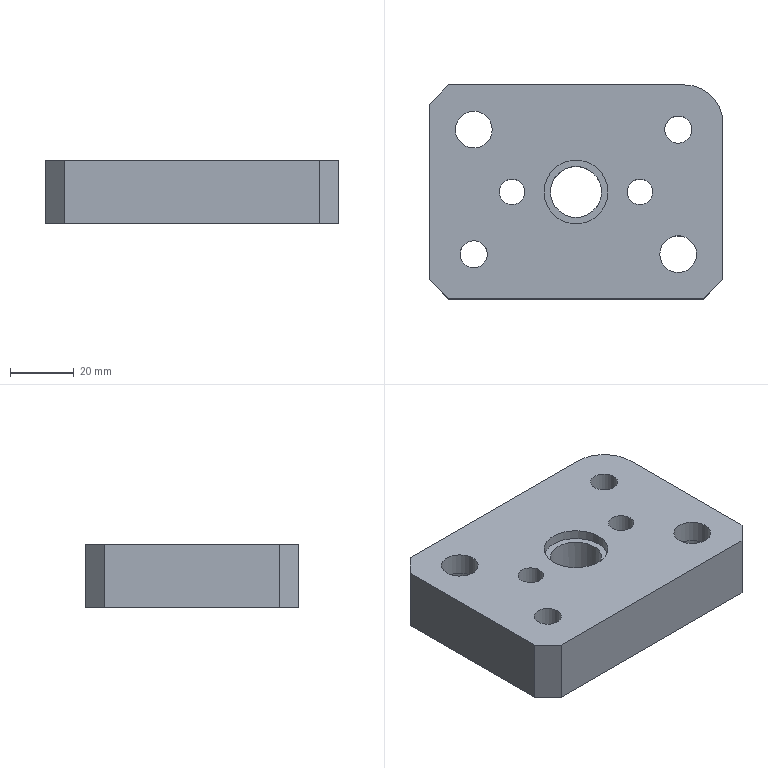Part | STEP file | lll_id594_x_t | 1 solid | 23 faces | box 92 x 67 x 20 mm | volume 104861 mm3 | plane 12 | cylinder 11 | commonest cylinder face diameters 8 x2 8.505 x2 11.509 x2 18.007 x2 16 x1 20 x1
STEP:
#1=CARTESIAN_POINT('',(994.747,-319.5,2.5));
#2=VERTEX_POINT('',#1);
#3=CARTESIAN_POINT('',(999.,-319.5,2.5));
#4=DIRECTION('',(0.,0.,-1.));
#5=DIRECTION('',(-1.,0.,0.));
#6=AXIS2_PLACEMENT_3D('',#3,#4,#5);
#7=CIRCLE('',#6,4.253);
#8=EDGE_CURVE('',#2,#2,#7,.T.);
#9=ORIENTED_EDGE('',*,*,#8,.F.);
#10=EDGE_LOOP('',(#9));
#11=FACE_BOUND('',#10,.T.);
#12=CARTESIAN_POINT('',(1072.003,-319.5,2.5));
#13=VERTEX_POINT('',#12);
#14=CARTESIAN_POINT('',(1063.,-319.5,2.5));
#15=DIRECTION('',(0.,0.,1.));
#16=DIRECTION('',(1.,0.,0.));
#17=AXIS2_PLACEMENT_3D('',#14,#15,#16);
#18=CIRCLE('',#17,9.004);
#19=EDGE_CURVE('',#13,#13,#18,.T.);
#20=ORIENTED_EDGE('',*,*,#19,.T.);
#21=EDGE_LOOP('',(#20));
#22=FACE_BOUND('',#21,.T.);
#23=CARTESIAN_POINT('',(1023.,-300.,2.5));
#24=VERTEX_POINT('',#23);
#25=CARTESIAN_POINT('',(1031.,-300.,2.5));
#26=DIRECTION('',(0.,0.,-1.));
#27=DIRECTION('',(-1.,0.,0.));
#28=AXIS2_PLACEMENT_3D('',#25,#26,#27);
#29=CIRCLE('',#28,8.);
#30=EDGE_CURVE('',#24,#24,#29,.T.);
#31=ORIENTED_EDGE('',*,*,#30,.F.);
#32=EDGE_LOOP('',(#31));
#33=FACE_BOUND('',#32,.T.);
#34=CARTESIAN_POINT('',(1047.,-300.,2.5));
#35=VERTEX_POINT('',#34);
#36=CARTESIAN_POINT('',(1051.,-300.,2.5));
#37=DIRECTION('',(0.,0.,-1.));
#38=DIRECTION('',(-1.,0.,0.));
#39=AXIS2_PLACEMENT_3D('',#36,#37,#38);
#40=CIRCLE('',#39,4.);
#41=EDGE_CURVE('',#35,#35,#40,.T.);
#42=ORIENTED_EDGE('',*,*,#41,.F.);
#43=EDGE_LOOP('',(#42));
#44=FACE_BOUND('',#43,.T.);
#45=CARTESIAN_POINT('',(1007.,-300.,2.5));
#46=VERTEX_POINT('',#45);
#47=CARTESIAN_POINT('',(1011.,-300.,2.5));
#48=DIRECTION('',(0.,0.,-1.));
#49=DIRECTION('',(-1.,0.,0.));
#50=AXIS2_PLACEMENT_3D('',#47,#48,#49);
#51=CIRCLE('',#50,4.);
#52=EDGE_CURVE('',#46,#46,#51,.T.);
#53=ORIENTED_EDGE('',*,*,#52,.F.);
#54=EDGE_LOOP('',(#53));
#55=FACE_BOUND('',#54,.T.);
#56=CARTESIAN_POINT('',(1065.,-266.5,2.5));
#57=VERTEX_POINT('',#56);
#58=CARTESIAN_POINT('',(991.,-266.5,2.5));
#59=VERTEX_POINT('',#58);
#60=CARTESIAN_POINT('',(1031.,-266.5,2.5));
#61=DIRECTION('',(-1.,0.,0.));
#62=VECTOR('',#61,1.);
#63=LINE('',#60,#62);
#64=EDGE_CURVE('',#57,#59,#63,.T.);
#65=ORIENTED_EDGE('',*,*,#64,.F.);
#66=CARTESIAN_POINT('',(1077.,-278.5,2.5));
#67=VERTEX_POINT('',#66);
#68=CARTESIAN_POINT('',(1065.,-278.5,2.5));
#69=DIRECTION('',(0.,0.,-1.));
#70=DIRECTION('',(-1.,0.,0.));
#71=AXIS2_PLACEMENT_3D('',#68,#69,#70);
#72=CIRCLE('',#71,12.);
#73=EDGE_CURVE('',#57,#67,#72,.T.);
#74=ORIENTED_EDGE('',*,*,#73,.T.);
#75=CARTESIAN_POINT('',(1077.,-327.5,2.5));
#76=VERTEX_POINT('',#75);
#77=CARTESIAN_POINT('',(1077.,-300.,2.5));
#78=DIRECTION('',(0.,1.,0.));
#79=VECTOR('',#78,1.);
#80=LINE('',#77,#79);
#81=EDGE_CURVE('',#76,#67,#80,.T.);
#82=ORIENTED_EDGE('',*,*,#81,.F.);
#83=CARTESIAN_POINT('',(1071.,-333.5,2.5));
#84=VERTEX_POINT('',#83);
#85=CARTESIAN_POINT('',(915.125,-489.375,2.5));
#86=DIRECTION('',(-0.7071,-0.7071,0.));
#87=VECTOR('',#86,1.);
#88=LINE('',#85,#87);
#89=EDGE_CURVE('',#76,#84,#88,.T.);
#90=ORIENTED_EDGE('',*,*,#89,.T.);
#91=CARTESIAN_POINT('',(991.,-333.5,2.5));
#92=VERTEX_POINT('',#91);
#93=CARTESIAN_POINT('',(1031.,-333.5,2.5));
#94=DIRECTION('',(1.,0.,0.));
#95=VECTOR('',#94,1.);
#96=LINE('',#93,#95);
#97=EDGE_CURVE('',#92,#84,#96,.T.);
#98=ORIENTED_EDGE('',*,*,#97,.F.);
#99=CARTESIAN_POINT('',(985.,-327.5,2.5));
#100=VERTEX_POINT('',#99);
#101=CARTESIAN_POINT('',(849.875,-192.375,2.5));
#102=DIRECTION('',(-0.7071,0.7071,0.));
#103=VECTOR('',#102,1.);
#104=LINE('',#101,#103);
#105=EDGE_CURVE('',#92,#100,#104,.T.);
#106=ORIENTED_EDGE('',*,*,#105,.T.);
#107=CARTESIAN_POINT('',(985.,-272.5,2.5));
#108=VERTEX_POINT('',#107);
#109=CARTESIAN_POINT('',(985.,-300.,2.5));
#110=DIRECTION('',(0.,-1.,0.));
#111=VECTOR('',#110,1.);
#112=LINE('',#109,#111);
#113=EDGE_CURVE('',#108,#100,#112,.T.);
#114=ORIENTED_EDGE('',*,*,#113,.F.);
#115=CARTESIAN_POINT('',(841.625,-415.875,2.5));
#116=DIRECTION('',(0.7071,0.7071,0.));
#117=VECTOR('',#116,1.);
#118=LINE('',#115,#117);
#119=EDGE_CURVE('',#108,#59,#118,.T.);
#120=ORIENTED_EDGE('',*,*,#119,.T.);
#121=EDGE_LOOP('',(#65,#74,#82,#90,#98,#106,#114,#120));
#122=FACE_BOUND('',#121,.T.);
#123=CARTESIAN_POINT('',(1058.747,-280.5,2.5));
#124=VERTEX_POINT('',#123);
#125=CARTESIAN_POINT('',(1063.,-280.5,2.5));
#126=DIRECTION('',(0.,0.,-1.));
#127=DIRECTION('',(-1.,0.,0.));
#128=AXIS2_PLACEMENT_3D('',#125,#126,#127);
#129=CIRCLE('',#128,4.253);
#130=EDGE_CURVE('',#124,#124,#129,.T.);
#131=ORIENTED_EDGE('',*,*,#130,.F.);
#132=EDGE_LOOP('',(#131));
#133=FACE_BOUND('',#132,.T.);
#134=CARTESIAN_POINT('',(1008.003,-280.5,2.5));
#135=VERTEX_POINT('',#134);
#136=CARTESIAN_POINT('',(999.,-280.5,2.5));
#137=DIRECTION('',(0.,0.,1.));
#138=DIRECTION('',(1.,0.,0.));
#139=AXIS2_PLACEMENT_3D('',#136,#137,#138);
#140=CIRCLE('',#139,9.004);
#141=EDGE_CURVE('',#135,#135,#140,.T.);
#142=ORIENTED_EDGE('',*,*,#141,.T.);
#143=EDGE_LOOP('',(#142));
#144=FACE_BOUND('',#143,.T.);
#145=CARTESIAN_POINT('',(734.,-308.25,2.5));
#146=DIRECTION('',(0.,0.,-1.));
#147=DIRECTION('',(1.,0.,0.));
#148=AXIS2_PLACEMENT_3D('',#145,#146,#147);
#149=PLANE('',#148);
#150=ADVANCED_FACE('',(#11,#22,#33,#44,#55,#122,#133,#144),#149,.T.);
#151=CARTESIAN_POINT('',(1003.252,-319.5,22.5));
#152=VERTEX_POINT('',#151);
#153=CARTESIAN_POINT('',(999.,-319.5,22.5));
#154=DIRECTION('',(0.,0.,1.));
#155=DIRECTION('',(1.,0.,0.));
#156=AXIS2_PLACEMENT_3D('',#153,#154,#155);
#157=CIRCLE('',#156,4.253);
#158=EDGE_CURVE('',#152,#152,#157,.T.);
#159=ORIENTED_EDGE('',*,*,#158,.F.);
#160=EDGE_LOOP('',(#159));
#161=FACE_BOUND('',#160,.T.);
#162=CARTESIAN_POINT('',(1004.754,-280.5,22.5));
#163=VERTEX_POINT('',#162);
#164=CARTESIAN_POINT('',(999.,-280.5,22.5));
#165=DIRECTION('',(0.,0.,1.));
#166=DIRECTION('',(1.,0.,0.));
#167=AXIS2_PLACEMENT_3D('',#164,#165,#166);
#168=CIRCLE('',#167,5.755);
#169=EDGE_CURVE('',#163,#163,#168,.T.);
#170=ORIENTED_EDGE('',*,*,#169,.F.);
#171=EDGE_LOOP('',(#170));
#172=FACE_BOUND('',#171,.T.);
#173=CARTESIAN_POINT('',(1067.252,-280.5,22.5));
#174=VERTEX_POINT('',#173);
#175=CARTESIAN_POINT('',(1063.,-280.5,22.5));
#176=DIRECTION('',(0.,0.,1.));
#177=DIRECTION('',(1.,0.,0.));
#178=AXIS2_PLACEMENT_3D('',#175,#176,#177);
#179=CIRCLE('',#178,4.253);
#180=EDGE_CURVE('',#174,#174,#179,.T.);
#181=ORIENTED_EDGE('',*,*,#180,.F.);
#182=EDGE_LOOP('',(#181));
#183=FACE_BOUND('',#182,.T.);
#184=CARTESIAN_POINT('',(1068.754,-319.5,22.5));
#185=VERTEX_POINT('',#184);
#186=CARTESIAN_POINT('',(1063.,-319.5,22.5));
#187=DIRECTION('',(0.,0.,1.));
#188=DIRECTION('',(1.,0.,0.));
#189=AXIS2_PLACEMENT_3D('',#186,#187,#188);
#190=CIRCLE('',#189,5.755);
#191=EDGE_CURVE('',#185,#185,#190,.T.);
#192=ORIENTED_EDGE('',*,*,#191,.F.);
#193=EDGE_LOOP('',(#192));
#194=FACE_BOUND('',#193,.T.);
#195=CARTESIAN_POINT('',(1077.,-278.5,22.5));
#196=VERTEX_POINT('',#195);
#197=CARTESIAN_POINT('',(1077.,-327.5,22.5));
#198=VERTEX_POINT('',#197);
#199=CARTESIAN_POINT('',(1077.,-300.,22.5));
#200=DIRECTION('',(0.,-1.,0.));
#201=VECTOR('',#200,1.);
#202=LINE('',#199,#201);
#203=EDGE_CURVE('',#196,#198,#202,.T.);
#204=ORIENTED_EDGE('',*,*,#203,.F.);
#205=CARTESIAN_POINT('',(1065.,-266.5,22.5));
#206=VERTEX_POINT('',#205);
#207=CARTESIAN_POINT('',(1065.,-278.5,22.5));
#208=DIRECTION('',(0.,0.,1.));
#209=DIRECTION('',(1.,0.,0.));
#210=AXIS2_PLACEMENT_3D('',#207,#208,#209);
#211=CIRCLE('',#210,12.);
#212=EDGE_CURVE('',#196,#206,#211,.T.);
#213=ORIENTED_EDGE('',*,*,#212,.T.);
#214=CARTESIAN_POINT('',(991.,-266.5,22.5));
#215=VERTEX_POINT('',#214);
#216=CARTESIAN_POINT('',(1031.,-266.5,22.5));
#217=DIRECTION('',(1.,0.,0.));
#218=VECTOR('',#217,1.);
#219=LINE('',#216,#218);
#220=EDGE_CURVE('',#215,#206,#219,.T.);
#221=ORIENTED_EDGE('',*,*,#220,.F.);
#222=CARTESIAN_POINT('',(985.,-272.5,22.5));
#223=VERTEX_POINT('',#222);
#224=CARTESIAN_POINT('',(841.625,-415.875,22.5));
#225=DIRECTION('',(-0.7071,-0.7071,0.));
#226=VECTOR('',#225,1.);
#227=LINE('',#224,#226);
#228=EDGE_CURVE('',#215,#223,#227,.T.);
#229=ORIENTED_EDGE('',*,*,#228,.T.);
#230=CARTESIAN_POINT('',(985.,-327.5,22.5));
#231=VERTEX_POINT('',#230);
#232=CARTESIAN_POINT('',(985.,-300.,22.5));
#233=DIRECTION('',(0.,1.,0.));
#234=VECTOR('',#233,1.);
#235=LINE('',#232,#234);
#236=EDGE_CURVE('',#231,#223,#235,.T.);
#237=ORIENTED_EDGE('',*,*,#236,.F.);
#238=CARTESIAN_POINT('',(991.,-333.5,22.5));
#239=VERTEX_POINT('',#238);
#240=CARTESIAN_POINT('',(849.875,-192.375,22.5));
#241=DIRECTION('',(0.7071,-0.7071,0.));
#242=VECTOR('',#241,1.);
#243=LINE('',#240,#242);
#244=EDGE_CURVE('',#231,#239,#243,.T.);
#245=ORIENTED_EDGE('',*,*,#244,.T.);
#246=CARTESIAN_POINT('',(1071.,-333.5,22.5));
#247=VERTEX_POINT('',#246);
#248=CARTESIAN_POINT('',(1031.,-333.5,22.5));
#249=DIRECTION('',(-1.,0.,0.));
#250=VECTOR('',#249,1.);
#251=LINE('',#248,#250);
#252=EDGE_CURVE('',#247,#239,#251,.T.);
#253=ORIENTED_EDGE('',*,*,#252,.F.);
#254=CARTESIAN_POINT('',(915.125,-489.375,22.5));
#255=DIRECTION('',(0.7071,0.7071,0.));
#256=VECTOR('',#255,1.);
#257=LINE('',#254,#256);
#258=EDGE_CURVE('',#247,#198,#257,.T.);
#259=ORIENTED_EDGE('',*,*,#258,.T.);
#260=EDGE_LOOP('',(#204,#213,#221,#229,#237,#245,#253,#259));
#261=FACE_BOUND('',#260,.T.);
#262=CARTESIAN_POINT('',(1041.,-300.,22.5));
#263=VERTEX_POINT('',#262);
#264=CARTESIAN_POINT('',(1031.,-300.,22.5));
#265=DIRECTION('',(0.,0.,-1.));
#266=DIRECTION('',(1.,0.,0.));
#267=AXIS2_PLACEMENT_3D('',#264,#265,#266);
#268=CIRCLE('',#267,10.);
#269=EDGE_CURVE('',#263,#263,#268,.T.);
#270=ORIENTED_EDGE('',*,*,#269,.T.);
#271=EDGE_LOOP('',(#270));
#272=FACE_BOUND('',#271,.T.);
#273=CARTESIAN_POINT('',(1015.,-300.,22.5));
#274=VERTEX_POINT('',#273);
#275=CARTESIAN_POINT('',(1011.,-300.,22.5));
#276=DIRECTION('',(0.,0.,1.));
#277=DIRECTION('',(1.,0.,0.));
#278=AXIS2_PLACEMENT_3D('',#275,#276,#277);
#279=CIRCLE('',#278,4.);
#280=EDGE_CURVE('',#274,#274,#279,.T.);
#281=ORIENTED_EDGE('',*,*,#280,.F.);
#282=EDGE_LOOP('',(#281));
#283=FACE_BOUND('',#282,.T.);
#284=CARTESIAN_POINT('',(1055.,-300.,22.5));
#285=VERTEX_POINT('',#284);
#286=CARTESIAN_POINT('',(1051.,-300.,22.5));
#287=DIRECTION('',(0.,0.,1.));
#288=DIRECTION('',(1.,0.,0.));
#289=AXIS2_PLACEMENT_3D('',#286,#287,#288);
#290=CIRCLE('',#289,4.);
#291=EDGE_CURVE('',#285,#285,#290,.T.);
#292=ORIENTED_EDGE('',*,*,#291,.F.);
#293=EDGE_LOOP('',(#292));
#294=FACE_BOUND('',#293,.T.);
#295=CARTESIAN_POINT('',(734.,-308.25,22.5));
#296=DIRECTION('',(0.,0.,1.));
#297=DIRECTION('',(-1.,0.,0.));
#298=AXIS2_PLACEMENT_3D('',#295,#296,#297);
#299=PLANE('',#298);
#300=ADVANCED_FACE('',(#161,#172,#183,#194,#261,#272,#283,#294),#299,.T.);
#301=ORIENTED_EDGE('',*,*,#81,.T.);
#302=CARTESIAN_POINT('',(1077.,-278.5,-36.5));
#303=DIRECTION('',(0.,0.,1.));
#304=VECTOR('',#303,1.);
#305=LINE('',#302,#304);
#306=EDGE_CURVE('',#67,#196,#305,.T.);
#307=ORIENTED_EDGE('',*,*,#306,.T.);
#308=ORIENTED_EDGE('',*,*,#203,.T.);
#309=CARTESIAN_POINT('',(1077.,-327.5,-36.5));
#310=DIRECTION('',(0.,0.,-1.));
#311=VECTOR('',#310,1.);
#312=LINE('',#309,#311);
#313=EDGE_CURVE('',#198,#76,#312,.T.);
#314=ORIENTED_EDGE('',*,*,#313,.T.);
#315=EDGE_LOOP('',(#301,#307,#308,#314));
#316=FACE_OUTER_BOUND('',#315,.T.);
#317=CARTESIAN_POINT('',(1077.,-300.,-36.5));
#318=DIRECTION('',(1.,0.,0.));
#319=DIRECTION('',(0.,0.,-1.));
#320=AXIS2_PLACEMENT_3D('',#317,#318,#319);
#321=PLANE('',#320);
#322=ADVANCED_FACE('',(#316),#321,.T.);
#323=ORIENTED_EDGE('',*,*,#252,.T.);
#324=CARTESIAN_POINT('',(991.,-333.5,-36.5));
#325=DIRECTION('',(0.,0.,-1.));
#326=VECTOR('',#325,1.);
#327=LINE('',#324,#326);
#328=EDGE_CURVE('',#239,#92,#327,.T.);
#329=ORIENTED_EDGE('',*,*,#328,.T.);
#330=ORIENTED_EDGE('',*,*,#97,.T.);
#331=CARTESIAN_POINT('',(1071.,-333.5,-36.5));
#332=DIRECTION('',(0.,0.,1.));
#333=VECTOR('',#332,1.);
#334=LINE('',#331,#333);
#335=EDGE_CURVE('',#84,#247,#334,.T.);
#336=ORIENTED_EDGE('',*,*,#335,.T.);
#337=EDGE_LOOP('',(#323,#329,#330,#336));
#338=FACE_OUTER_BOUND('',#337,.T.);
#339=CARTESIAN_POINT('',(1031.,-333.5,-36.5));
#340=DIRECTION('',(0.,-1.,0.));
#341=DIRECTION('',(0.,0.,-1.));
#342=AXIS2_PLACEMENT_3D('',#339,#340,#341);
#343=PLANE('',#342);
#344=ADVANCED_FACE('',(#338),#343,.T.);
#345=ORIENTED_EDGE('',*,*,#113,.T.);
#346=CARTESIAN_POINT('',(985.,-327.5,-36.5));
#347=DIRECTION('',(0.,0.,1.));
#348=VECTOR('',#347,1.);
#349=LINE('',#346,#348);
#350=EDGE_CURVE('',#100,#231,#349,.T.);
#351=ORIENTED_EDGE('',*,*,#350,.T.);
#352=ORIENTED_EDGE('',*,*,#236,.T.);
#353=CARTESIAN_POINT('',(985.,-272.5,-36.5));
#354=DIRECTION('',(0.,0.,-1.));
#355=VECTOR('',#354,1.);
#356=LINE('',#353,#355);
#357=EDGE_CURVE('',#223,#108,#356,.T.);
#358=ORIENTED_EDGE('',*,*,#357,.T.);
#359=EDGE_LOOP('',(#345,#351,#352,#358));
#360=FACE_OUTER_BOUND('',#359,.T.);
#361=CARTESIAN_POINT('',(985.,-300.,-36.5));
#362=DIRECTION('',(-1.,0.,0.));
#363=DIRECTION('',(0.,0.,1.));
#364=AXIS2_PLACEMENT_3D('',#361,#362,#363);
#365=PLANE('',#364);
#366=ADVANCED_FACE('',(#360),#365,.T.);
#367=ORIENTED_EDGE('',*,*,#220,.T.);
#368=CARTESIAN_POINT('',(1065.,-266.5,-36.5));
#369=DIRECTION('',(0.,0.,-1.));
#370=VECTOR('',#369,1.);
#371=LINE('',#368,#370);
#372=EDGE_CURVE('',#206,#57,#371,.T.);
#373=ORIENTED_EDGE('',*,*,#372,.T.);
#374=ORIENTED_EDGE('',*,*,#64,.T.);
#375=CARTESIAN_POINT('',(991.,-266.5,-36.5));
#376=DIRECTION('',(0.,0.,1.));
#377=VECTOR('',#376,1.);
#378=LINE('',#375,#377);
#379=EDGE_CURVE('',#59,#215,#378,.T.);
#380=ORIENTED_EDGE('',*,*,#379,.T.);
#381=EDGE_LOOP('',(#367,#373,#374,#380));
#382=FACE_OUTER_BOUND('',#381,.T.);
#383=CARTESIAN_POINT('',(1031.,-266.5,-36.5));
#384=DIRECTION('',(0.,1.,0.));
#385=DIRECTION('',(0.,0.,1.));
#386=AXIS2_PLACEMENT_3D('',#383,#384,#385);
#387=PLANE('',#386);
#388=ADVANCED_FACE('',(#382),#387,.T.);
#389=ORIENTED_EDGE('',*,*,#52,.T.);
#390=EDGE_LOOP('',(#389));
#391=FACE_BOUND('',#390,.T.);
#392=ORIENTED_EDGE('',*,*,#280,.T.);
#393=EDGE_LOOP('',(#392));
#394=FACE_BOUND('',#393,.T.);
#395=CARTESIAN_POINT('',(1011.,-300.,19.5));
#396=DIRECTION('',(0.,0.,-1.));
#397=DIRECTION('',(0.,1.,0.));
#398=AXIS2_PLACEMENT_3D('',#395,#396,#397);
#399=CYLINDRICAL_SURFACE('',#398,4.);
#400=ADVANCED_FACE('',(#391,#394),#399,.F.);
#401=ORIENTED_EDGE('',*,*,#41,.T.);
#402=EDGE_LOOP('',(#401));
#403=FACE_BOUND('',#402,.T.);
#404=ORIENTED_EDGE('',*,*,#291,.T.);
#405=EDGE_LOOP('',(#404));
#406=FACE_BOUND('',#405,.T.);
#407=CARTESIAN_POINT('',(1051.,-300.,19.5));
#408=DIRECTION('',(0.,0.,-1.));
#409=DIRECTION('',(0.,-1.,0.));
#410=AXIS2_PLACEMENT_3D('',#407,#408,#409);
#411=CYLINDRICAL_SURFACE('',#410,4.);
#412=ADVANCED_FACE('',(#403,#406),#411,.F.);
#413=CARTESIAN_POINT('',(1021.,-300.,19.5));
#414=VERTEX_POINT('',#413);
#415=CARTESIAN_POINT('',(1031.,-300.,19.5));
#416=DIRECTION('',(0.,0.,-1.));
#417=DIRECTION('',(-1.,0.,0.));
#418=AXIS2_PLACEMENT_3D('',#415,#416,#417);
#419=CIRCLE('',#418,10.);
#420=EDGE_CURVE('',#414,#414,#419,.T.);
#421=ORIENTED_EDGE('',*,*,#420,.T.);
#422=EDGE_LOOP('',(#421));
#423=FACE_BOUND('',#422,.T.);
#424=ORIENTED_EDGE('',*,*,#269,.F.);
#425=EDGE_LOOP('',(#424));
#426=FACE_BOUND('',#425,.T.);
#427=CARTESIAN_POINT('',(1031.,-300.,22.5));
#428=DIRECTION('',(0.,0.,-1.));
#429=DIRECTION('',(0.,1.,0.));
#430=AXIS2_PLACEMENT_3D('',#427,#428,#429);
#431=CYLINDRICAL_SURFACE('',#430,10.);
#432=ADVANCED_FACE('',(#423,#426),#431,.F.);
#433=CARTESIAN_POINT('',(1031.,-292.,19.5));
#434=VERTEX_POINT('',#433);
#435=CARTESIAN_POINT('',(1031.,-300.,19.5));
#436=DIRECTION('',(0.,0.,1.));
#437=DIRECTION('',(0.,1.,0.));
#438=AXIS2_PLACEMENT_3D('',#435,#436,#437);
#439=CIRCLE('',#438,8.);
#440=EDGE_CURVE('',#434,#434,#439,.T.);
#441=ORIENTED_EDGE('',*,*,#440,.F.);
#442=EDGE_LOOP('',(#441));
#443=FACE_BOUND('',#442,.T.);
#444=ORIENTED_EDGE('',*,*,#420,.F.);
#445=EDGE_LOOP('',(#444));
#446=FACE_BOUND('',#445,.T.);
#447=CARTESIAN_POINT('',(1031.,-300.,19.5));
#448=DIRECTION('',(0.,0.,-1.));
#449=DIRECTION('',(0.,1.,0.));
#450=AXIS2_PLACEMENT_3D('',#447,#448,#449);
#451=PLANE('',#450);
#452=ADVANCED_FACE('',(#443,#446),#451,.F.);
#453=ORIENTED_EDGE('',*,*,#30,.T.);
#454=EDGE_LOOP('',(#453));
#455=FACE_BOUND('',#454,.T.);
#456=ORIENTED_EDGE('',*,*,#440,.T.);
#457=EDGE_LOOP('',(#456));
#458=FACE_BOUND('',#457,.T.);
#459=CARTESIAN_POINT('',(1031.,-300.,15.5));
#460=DIRECTION('',(0.,0.,-1.));
#461=DIRECTION('',(0.,1.,0.));
#462=AXIS2_PLACEMENT_3D('',#459,#460,#461);
#463=CYLINDRICAL_SURFACE('',#462,8.);
#464=ADVANCED_FACE('',(#455,#458),#463,.F.);
#465=ORIENTED_EDGE('',*,*,#191,.T.);
#466=EDGE_LOOP('',(#465));
#467=FACE_BOUND('',#466,.T.);
#468=CARTESIAN_POINT('',(1068.754,-319.5,15.5));
#469=VERTEX_POINT('',#468);
#470=CARTESIAN_POINT('',(1063.,-319.5,15.5));
#471=DIRECTION('',(0.,0.,1.));
#472=DIRECTION('',(1.,0.,0.));
#473=AXIS2_PLACEMENT_3D('',#470,#471,#472);
#474=CIRCLE('',#473,5.755);
#475=EDGE_CURVE('',#469,#469,#474,.T.);
#476=ORIENTED_EDGE('',*,*,#475,.F.);
#477=EDGE_LOOP('',(#476));
#478=FACE_BOUND('',#477,.T.);
#479=CARTESIAN_POINT('',(1063.,-319.5,-2.5));
#480=DIRECTION('',(0.,0.,1.));
#481=DIRECTION('',(1.,0.,0.));
#482=AXIS2_PLACEMENT_3D('',#479,#480,#481);
#483=CYLINDRICAL_SURFACE('',#482,5.755);
#484=ADVANCED_FACE('',(#467,#478),#483,.F.);
#485=ORIENTED_EDGE('',*,*,#475,.T.);
#486=EDGE_LOOP('',(#485));
#487=FACE_BOUND('',#486,.T.);
#488=CARTESIAN_POINT('',(1072.003,-319.5,15.5));
#489=VERTEX_POINT('',#488);
#490=CARTESIAN_POINT('',(1063.,-319.5,15.5));
#491=DIRECTION('',(0.,0.,1.));
#492=DIRECTION('',(1.,0.,0.));
#493=AXIS2_PLACEMENT_3D('',#490,#491,#492);
#494=CIRCLE('',#493,9.004);
#495=EDGE_CURVE('',#489,#489,#494,.T.);
#496=ORIENTED_EDGE('',*,*,#495,.F.);
#497=EDGE_LOOP('',(#496));
#498=FACE_BOUND('',#497,.T.);
#499=CARTESIAN_POINT('',(1063.,-319.5,15.5));
#500=DIRECTION('',(0.,0.,1.));
#501=DIRECTION('',(1.,0.,0.));
#502=AXIS2_PLACEMENT_3D('',#499,#500,#501);
#503=PLANE('',#502);
#504=ADVANCED_FACE('',(#487,#498),#503,.F.);
#505=ORIENTED_EDGE('',*,*,#495,.T.);
#506=EDGE_LOOP('',(#505));
#507=FACE_BOUND('',#506,.T.);
#508=ORIENTED_EDGE('',*,*,#19,.F.);
#509=EDGE_LOOP('',(#508));
#510=FACE_BOUND('',#509,.T.);
#511=CARTESIAN_POINT('',(1063.,-319.5,2.5));
#512=DIRECTION('',(0.,0.,1.));
#513=DIRECTION('',(1.,0.,0.));
#514=AXIS2_PLACEMENT_3D('',#511,#512,#513);
#515=CYLINDRICAL_SURFACE('',#514,9.004);
#516=ADVANCED_FACE('',(#507,#510),#515,.F.);
#517=ORIENTED_EDGE('',*,*,#130,.T.);
#518=EDGE_LOOP('',(#517));
#519=FACE_BOUND('',#518,.T.);
#520=ORIENTED_EDGE('',*,*,#180,.T.);
#521=EDGE_LOOP('',(#520));
#522=FACE_BOUND('',#521,.T.);
#523=CARTESIAN_POINT('',(1063.,-280.5,-2.5));
#524=DIRECTION('',(0.,0.,1.));
#525=DIRECTION('',(1.,0.,0.));
#526=AXIS2_PLACEMENT_3D('',#523,#524,#525);
#527=CYLINDRICAL_SURFACE('',#526,4.253);
#528=ADVANCED_FACE('',(#519,#522),#527,.F.);
#529=ORIENTED_EDGE('',*,*,#169,.T.);
#530=EDGE_LOOP('',(#529));
#531=FACE_BOUND('',#530,.T.);
#532=CARTESIAN_POINT('',(1004.754,-280.5,15.5));
#533=VERTEX_POINT('',#532);
#534=CARTESIAN_POINT('',(999.,-280.5,15.5));
#535=DIRECTION('',(0.,0.,1.));
#536=DIRECTION('',(1.,0.,0.));
#537=AXIS2_PLACEMENT_3D('',#534,#535,#536);
#538=CIRCLE('',#537,5.755);
#539=EDGE_CURVE('',#533,#533,#538,.T.);
#540=ORIENTED_EDGE('',*,*,#539,.F.);
#541=EDGE_LOOP('',(#540));
#542=FACE_BOUND('',#541,.T.);
#543=CARTESIAN_POINT('',(999.,-280.5,-2.5));
#544=DIRECTION('',(0.,0.,1.));
#545=DIRECTION('',(1.,0.,0.));
#546=AXIS2_PLACEMENT_3D('',#543,#544,#545);
#547=CYLINDRICAL_SURFACE('',#546,5.755);
#548=ADVANCED_FACE('',(#531,#542),#547,.F.);
#549=ORIENTED_EDGE('',*,*,#539,.T.);
#550=EDGE_LOOP('',(#549));
#551=FACE_BOUND('',#550,.T.);
#552=CARTESIAN_POINT('',(1008.003,-280.5,15.5));
#553=VERTEX_POINT('',#552);
#554=CARTESIAN_POINT('',(999.,-280.5,15.5));
#555=DIRECTION('',(0.,0.,1.));
#556=DIRECTION('',(1.,0.,0.));
#557=AXIS2_PLACEMENT_3D('',#554,#555,#556);
#558=CIRCLE('',#557,9.004);
#559=EDGE_CURVE('',#553,#553,#558,.T.);
#560=ORIENTED_EDGE('',*,*,#559,.F.);
#561=EDGE_LOOP('',(#560));
#562=FACE_BOUND('',#561,.T.);
#563=CARTESIAN_POINT('',(999.,-280.5,15.5));
#564=DIRECTION('',(0.,0.,1.));
#565=DIRECTION('',(1.,0.,0.));
#566=AXIS2_PLACEMENT_3D('',#563,#564,#565);
#567=PLANE('',#566);
#568=ADVANCED_FACE('',(#551,#562),#567,.F.);
#569=ORIENTED_EDGE('',*,*,#559,.T.);
#570=EDGE_LOOP('',(#569));
#571=FACE_BOUND('',#570,.T.);
#572=ORIENTED_EDGE('',*,*,#141,.F.);
#573=EDGE_LOOP('',(#572));
#574=FACE_BOUND('',#573,.T.);
#575=CARTESIAN_POINT('',(999.,-280.5,2.5));
#576=DIRECTION('',(0.,0.,1.));
#577=DIRECTION('',(1.,0.,0.));
#578=AXIS2_PLACEMENT_3D('',#575,#576,#577);
#579=CYLINDRICAL_SURFACE('',#578,9.004);
#580=ADVANCED_FACE('',(#571,#574),#579,.F.);
#581=ORIENTED_EDGE('',*,*,#8,.T.);
#582=EDGE_LOOP('',(#581));
#583=FACE_BOUND('',#582,.T.);
#584=ORIENTED_EDGE('',*,*,#158,.T.);
#585=EDGE_LOOP('',(#584));
#586=FACE_BOUND('',#585,.T.);
#587=CARTESIAN_POINT('',(999.,-319.5,-2.5));
#588=DIRECTION('',(0.,0.,1.));
#589=DIRECTION('',(1.,0.,0.));
#590=AXIS2_PLACEMENT_3D('',#587,#588,#589);
#591=CYLINDRICAL_SURFACE('',#590,4.253);
#592=ADVANCED_FACE('',(#583,#586),#591,.F.);
#593=ORIENTED_EDGE('',*,*,#105,.F.);
#594=ORIENTED_EDGE('',*,*,#328,.F.);
#595=ORIENTED_EDGE('',*,*,#244,.F.);
#596=ORIENTED_EDGE('',*,*,#350,.F.);
#597=EDGE_LOOP('',(#593,#594,#595,#596));
#598=FACE_OUTER_BOUND('',#597,.T.);
#599=CARTESIAN_POINT('',(985.,-327.5,-36.5));
#600=DIRECTION('',(0.7071,0.7071,0.));
#601=DIRECTION('',(0.,0.,-1.));
#602=AXIS2_PLACEMENT_3D('',#599,#600,#601);
#603=PLANE('',#602);
#604=ADVANCED_FACE('',(#598),#603,.F.);
#605=ORIENTED_EDGE('',*,*,#119,.F.);
#606=ORIENTED_EDGE('',*,*,#357,.F.);
#607=ORIENTED_EDGE('',*,*,#228,.F.);
#608=ORIENTED_EDGE('',*,*,#379,.F.);
#609=EDGE_LOOP('',(#605,#606,#607,#608));
#610=FACE_OUTER_BOUND('',#609,.T.);
#611=CARTESIAN_POINT('',(991.,-266.5,-36.5));
#612=DIRECTION('',(0.7071,-0.7071,0.));
#613=DIRECTION('',(0.,0.,-1.));
#614=AXIS2_PLACEMENT_3D('',#611,#612,#613);
#615=PLANE('',#614);
#616=ADVANCED_FACE('',(#610),#615,.F.);
#617=ORIENTED_EDGE('',*,*,#89,.F.);
#618=ORIENTED_EDGE('',*,*,#313,.F.);
#619=ORIENTED_EDGE('',*,*,#258,.F.);
#620=ORIENTED_EDGE('',*,*,#335,.F.);
#621=EDGE_LOOP('',(#617,#618,#619,#620));
#622=FACE_OUTER_BOUND('',#621,.T.);
#623=CARTESIAN_POINT('',(1071.,-333.5,-36.5));
#624=DIRECTION('',(-0.7071,0.7071,0.));
#625=DIRECTION('',(0.,0.,-1.));
#626=AXIS2_PLACEMENT_3D('',#623,#624,#625);
#627=PLANE('',#626);
#628=ADVANCED_FACE('',(#622),#627,.F.);
#629=ORIENTED_EDGE('',*,*,#73,.F.);
#630=ORIENTED_EDGE('',*,*,#372,.F.);
#631=ORIENTED_EDGE('',*,*,#212,.F.);
#632=ORIENTED_EDGE('',*,*,#306,.F.);
#633=EDGE_LOOP('',(#629,#630,#631,#632));
#634=FACE_OUTER_BOUND('',#633,.T.);
#635=CARTESIAN_POINT('',(1065.,-278.5,-36.5));
#636=DIRECTION('',(0.,0.,1.));
#637=DIRECTION('',(-1.,0.,0.));
#638=AXIS2_PLACEMENT_3D('',#635,#636,#637);
#639=CYLINDRICAL_SURFACE('',#638,12.);
#640=ADVANCED_FACE('',(#634),#639,.T.);
#641=CLOSED_SHELL('',(#150,#300,#322,#344,#366,#388,#400,#412,#432,#452,#464,#484,#504,#516,#528,#548,#568,#580,#592,#604,#616,#628,#640));
#642=MANIFOLD_SOLID_BREP('',#641);
#643=(LENGTH_UNIT()NAMED_UNIT(*)SI_UNIT(.MILLI.,.METRE.));
#644=UNCERTAINTY_MEASURE_WITH_UNIT(LENGTH_MEASURE(0.00002),#643,'','');
#645=(NAMED_UNIT(*)PLANE_ANGLE_UNIT()SI_UNIT($,.RADIAN.));
#646=PLANE_ANGLE_MEASURE_WITH_UNIT(PLANE_ANGLE_MEASURE(0.01745),#645);
#647=DIMENSIONAL_EXPONENTS(0.,0.,0.,0.,0.,0.,0.);
#648=(CONVERSION_BASED_UNIT('DEGREE',#646)NAMED_UNIT(#647)PLANE_ANGLE_UNIT());
#649=(NAMED_UNIT(*)SI_UNIT($,.STERADIAN.)SOLID_ANGLE_UNIT());
#650=(GEOMETRIC_REPRESENTATION_CONTEXT(3)GLOBAL_UNCERTAINTY_ASSIGNED_CONTEXT((#644))GLOBAL_UNIT_ASSIGNED_CONTEXT((#643,#648,#649))REPRESENTATION_CONTEXT('',''));
#651=ADVANCED_BREP_SHAPE_REPRESENTATION('',(#642),#650);